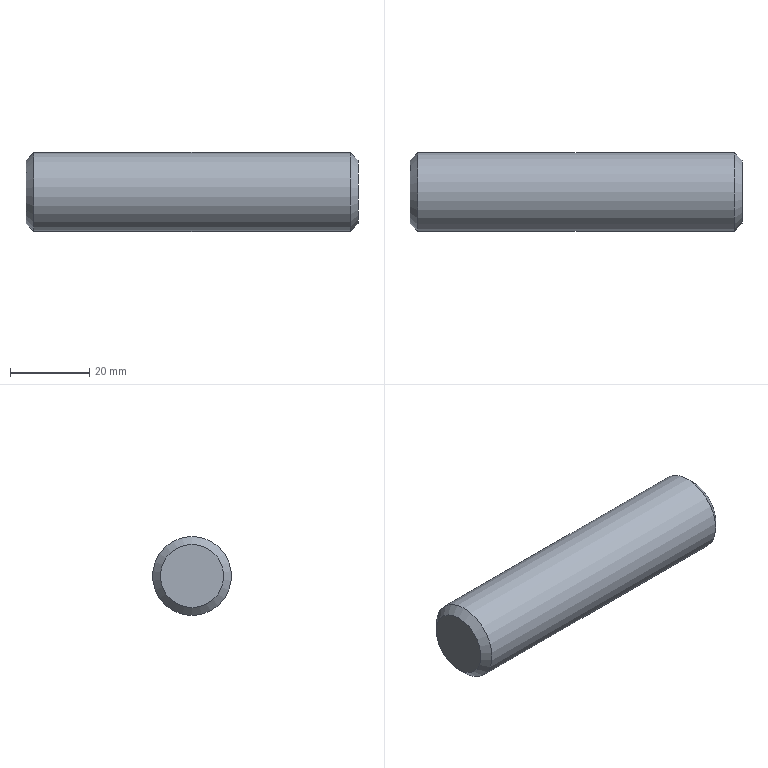Part | STEP file | solid 196 | 1 solid | 5 faces | box 84 x 20 x 20 mm | volume 26155 mm3 | plane 2 | cone 2 | cylinder 1 | commonest cylinder face diameters 20 x1